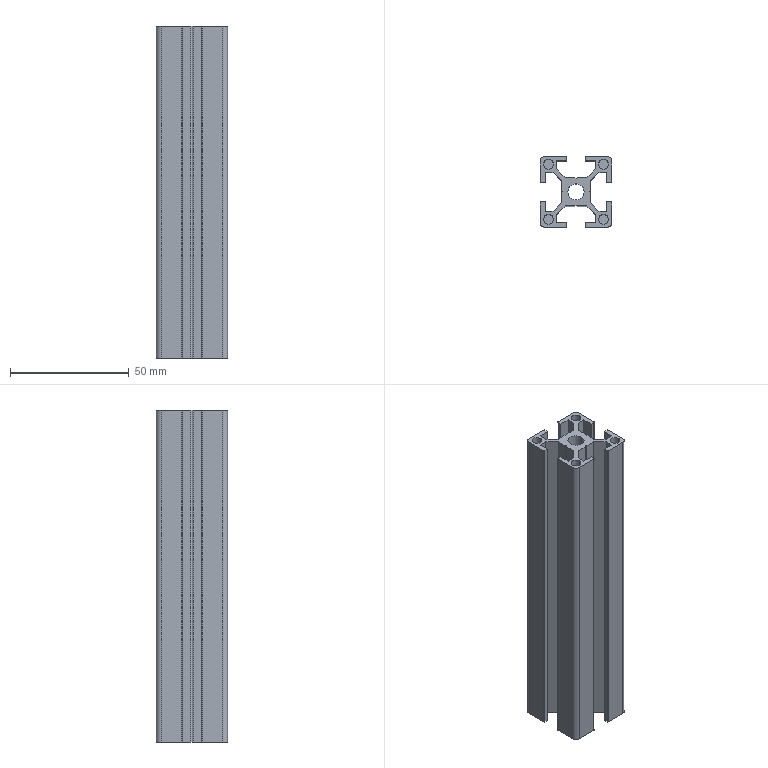Part | STEP file | SQ-8-3030W-160_Default | 1 solid | 84 faces | box 30 x 30 x 140 mm | volume 48663 mm3 | plane 62 | cylinder 22 | commonest cylinder face diameters 0.6 x8 4.2 x8 4 x4 6.8 x2